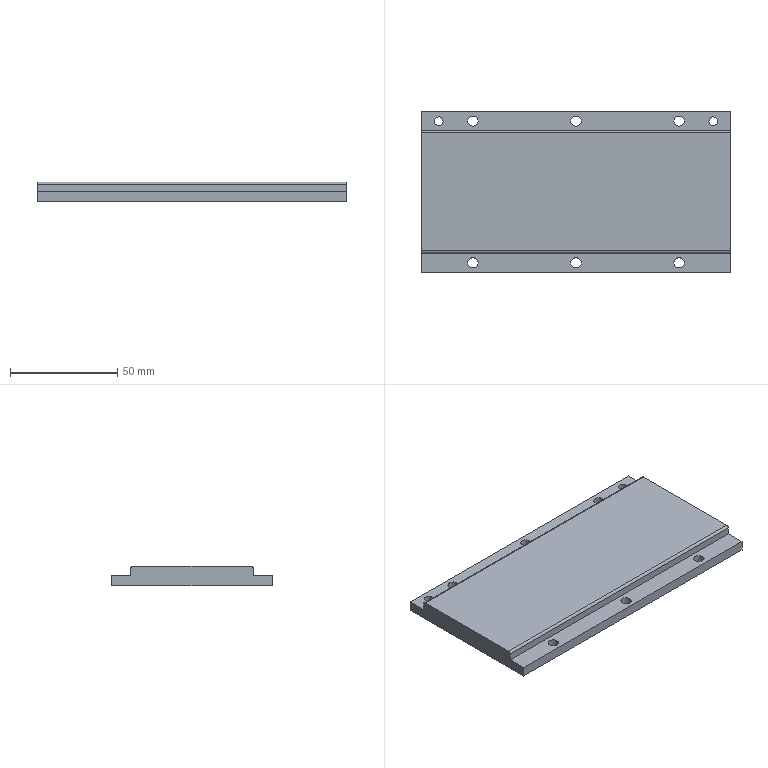Part | NX | features BREP 1 | 1 solid | 28 faces | box 143.8 x 75 x 9.2 mm | volume 87123 mm3 | cylinder 18 | plane 10 | commonest cylinder face diameters 4.8 x12 4.1 x4 2 x2
STEP:
#1=CARTESIAN_POINT('',(133.85,33.,2.4));
#2=VERTEX_POINT('',#1);
#3=CARTESIAN_POINT('',(133.85,33.,-2.4));
#4=VERTEX_POINT('',#3);
#5=CARTESIAN_POINT('',(133.85,33.,2.4));
#6=DIRECTION('',(0.,0.,1.));
#7=VECTOR('',#6,1000.);
#8=LINE('',#5,#7);
#9=EDGE_CURVE('',#2,#4,#8,.F.);
#10=ORIENTED_EDGE('',*,*,#9,.T.);
#11=CARTESIAN_POINT('',(137.95,33.,-2.4));
#12=VERTEX_POINT('',#11);
#13=CARTESIAN_POINT('',(135.9,33.,-2.4));
#14=DIRECTION('',(0.,0.,1.));
#15=DIRECTION('',(1.,0.,0.));
#16=AXIS2_PLACEMENT_3D('',#13,#14,#15);
#17=CIRCLE('',#16,2.05);
#18=EDGE_CURVE('',#12,#4,#17,.T.);
#19=ORIENTED_EDGE('',*,*,#18,.F.);
#20=CARTESIAN_POINT('',(137.95,33.,2.4));
#21=VERTEX_POINT('',#20);
#22=CARTESIAN_POINT('',(137.95,33.,2.4));
#23=DIRECTION('',(0.,0.,1.));
#24=VECTOR('',#23,1000.);
#25=LINE('',#22,#24);
#26=EDGE_CURVE('',#21,#12,#25,.F.);
#27=ORIENTED_EDGE('',*,*,#26,.F.);
#28=CARTESIAN_POINT('',(135.9,33.,2.4));
#29=DIRECTION('',(0.,0.,1.));
#30=DIRECTION('',(1.,0.,0.));
#31=AXIS2_PLACEMENT_3D('',#28,#29,#30);
#32=CIRCLE('',#31,2.05);
#33=EDGE_CURVE('',#21,#2,#32,.T.);
#34=ORIENTED_EDGE('',*,*,#33,.T.);
#35=EDGE_LOOP('',(#10,#19,#27,#34));
#36=FACE_BOUND('',#35,.T.);
#37=CARTESIAN_POINT('',(135.9,33.,2.4));
#38=DIRECTION('',(0.,0.,1.));
#39=DIRECTION('',(1.,0.,0.));
#40=AXIS2_PLACEMENT_3D('',#37,#38,#39);
#41=CYLINDRICAL_SURFACE('',#40,2.05);
#42=ADVANCED_FACE('',(#36),#41,.F.);
#43=CARTESIAN_POINT('',(5.85,33.,2.4));
#44=VERTEX_POINT('',#43);
#45=CARTESIAN_POINT('',(5.85,33.,-2.4));
#46=VERTEX_POINT('',#45);
#47=CARTESIAN_POINT('',(5.85,33.,2.4));
#48=DIRECTION('',(0.,0.,1.));
#49=VECTOR('',#48,1000.);
#50=LINE('',#47,#49);
#51=EDGE_CURVE('',#44,#46,#50,.F.);
#52=ORIENTED_EDGE('',*,*,#51,.T.);
#53=CARTESIAN_POINT('',(9.95,33.,-2.4));
#54=VERTEX_POINT('',#53);
#55=CARTESIAN_POINT('',(7.9,33.,-2.4));
#56=DIRECTION('',(0.,0.,1.));
#57=DIRECTION('',(1.,0.,0.));
#58=AXIS2_PLACEMENT_3D('',#55,#56,#57);
#59=CIRCLE('',#58,2.05);
#60=EDGE_CURVE('',#54,#46,#59,.T.);
#61=ORIENTED_EDGE('',*,*,#60,.F.);
#62=CARTESIAN_POINT('',(9.95,33.,2.4));
#63=VERTEX_POINT('',#62);
#64=CARTESIAN_POINT('',(9.95,33.,2.4));
#65=DIRECTION('',(0.,0.,1.));
#66=VECTOR('',#65,1000.);
#67=LINE('',#64,#66);
#68=EDGE_CURVE('',#63,#54,#67,.F.);
#69=ORIENTED_EDGE('',*,*,#68,.F.);
#70=CARTESIAN_POINT('',(7.9,33.,2.4));
#71=DIRECTION('',(0.,0.,1.));
#72=DIRECTION('',(1.,0.,0.));
#73=AXIS2_PLACEMENT_3D('',#70,#71,#72);
#74=CIRCLE('',#73,2.05);
#75=EDGE_CURVE('',#63,#44,#74,.T.);
#76=ORIENTED_EDGE('',*,*,#75,.T.);
#77=EDGE_LOOP('',(#52,#61,#69,#76));
#78=FACE_BOUND('',#77,.T.);
#79=CARTESIAN_POINT('',(7.9,33.,2.4));
#80=DIRECTION('',(0.,0.,1.));
#81=DIRECTION('',(1.,0.,0.));
#82=AXIS2_PLACEMENT_3D('',#79,#80,#81);
#83=CYLINDRICAL_SURFACE('',#82,2.05);
#84=ADVANCED_FACE('',(#78),#83,.F.);
#85=CARTESIAN_POINT('',(117.5,33.,2.4));
#86=VERTEX_POINT('',#85);
#87=CARTESIAN_POINT('',(117.5,33.,-2.4));
#88=VERTEX_POINT('',#87);
#89=CARTESIAN_POINT('',(117.5,33.,2.4));
#90=DIRECTION('',(0.,0.,1.));
#91=VECTOR('',#90,1000.);
#92=LINE('',#89,#91);
#93=EDGE_CURVE('',#86,#88,#92,.F.);
#94=ORIENTED_EDGE('',*,*,#93,.T.);
#95=CARTESIAN_POINT('',(122.3,33.,-2.4));
#96=VERTEX_POINT('',#95);
#97=CARTESIAN_POINT('',(119.9,33.,-2.4));
#98=DIRECTION('',(0.,0.,1.));
#99=DIRECTION('',(1.,0.,0.));
#100=AXIS2_PLACEMENT_3D('',#97,#98,#99);
#101=CIRCLE('',#100,2.4);
#102=EDGE_CURVE('',#96,#88,#101,.T.);
#103=ORIENTED_EDGE('',*,*,#102,.F.);
#104=CARTESIAN_POINT('',(122.3,33.,2.4));
#105=VERTEX_POINT('',#104);
#106=CARTESIAN_POINT('',(122.3,33.,2.4));
#107=DIRECTION('',(0.,0.,1.));
#108=VECTOR('',#107,1000.);
#109=LINE('',#106,#108);
#110=EDGE_CURVE('',#105,#96,#109,.F.);
#111=ORIENTED_EDGE('',*,*,#110,.F.);
#112=CARTESIAN_POINT('',(119.9,33.,2.4));
#113=DIRECTION('',(0.,0.,1.));
#114=DIRECTION('',(1.,0.,0.));
#115=AXIS2_PLACEMENT_3D('',#112,#113,#114);
#116=CIRCLE('',#115,2.4);
#117=EDGE_CURVE('',#105,#86,#116,.T.);
#118=ORIENTED_EDGE('',*,*,#117,.T.);
#119=EDGE_LOOP('',(#94,#103,#111,#118));
#120=FACE_BOUND('',#119,.T.);
#121=CARTESIAN_POINT('',(119.9,33.,2.4));
#122=DIRECTION('',(0.,0.,1.));
#123=DIRECTION('',(1.,0.,0.));
#124=AXIS2_PLACEMENT_3D('',#121,#122,#123);
#125=CYLINDRICAL_SURFACE('',#124,2.4);
#126=ADVANCED_FACE('',(#120),#125,.F.);
#127=CARTESIAN_POINT('',(117.5,-33.,2.4));
#128=VERTEX_POINT('',#127);
#129=CARTESIAN_POINT('',(117.5,-33.,-2.4));
#130=VERTEX_POINT('',#129);
#131=CARTESIAN_POINT('',(117.5,-33.,2.4));
#132=DIRECTION('',(0.,0.,1.));
#133=VECTOR('',#132,1000.);
#134=LINE('',#131,#133);
#135=EDGE_CURVE('',#128,#130,#134,.F.);
#136=ORIENTED_EDGE('',*,*,#135,.T.);
#137=CARTESIAN_POINT('',(122.3,-33.,-2.4));
#138=VERTEX_POINT('',#137);
#139=CARTESIAN_POINT('',(119.9,-33.,-2.4));
#140=DIRECTION('',(0.,0.,1.));
#141=DIRECTION('',(1.,0.,0.));
#142=AXIS2_PLACEMENT_3D('',#139,#140,#141);
#143=CIRCLE('',#142,2.4);
#144=EDGE_CURVE('',#138,#130,#143,.T.);
#145=ORIENTED_EDGE('',*,*,#144,.F.);
#146=CARTESIAN_POINT('',(122.3,-33.,2.4));
#147=VERTEX_POINT('',#146);
#148=CARTESIAN_POINT('',(122.3,-33.,2.4));
#149=DIRECTION('',(0.,0.,1.));
#150=VECTOR('',#149,1000.);
#151=LINE('',#148,#150);
#152=EDGE_CURVE('',#147,#138,#151,.F.);
#153=ORIENTED_EDGE('',*,*,#152,.F.);
#154=CARTESIAN_POINT('',(119.9,-33.,2.4));
#155=DIRECTION('',(0.,0.,1.));
#156=DIRECTION('',(1.,0.,0.));
#157=AXIS2_PLACEMENT_3D('',#154,#155,#156);
#158=CIRCLE('',#157,2.4);
#159=EDGE_CURVE('',#147,#128,#158,.T.);
#160=ORIENTED_EDGE('',*,*,#159,.T.);
#161=EDGE_LOOP('',(#136,#145,#153,#160));
#162=FACE_BOUND('',#161,.T.);
#163=CARTESIAN_POINT('',(119.9,-33.,2.4));
#164=DIRECTION('',(0.,0.,1.));
#165=DIRECTION('',(1.,0.,0.));
#166=AXIS2_PLACEMENT_3D('',#163,#164,#165);
#167=CYLINDRICAL_SURFACE('',#166,2.4);
#168=ADVANCED_FACE('',(#162),#167,.F.);
#169=CARTESIAN_POINT('',(69.5,33.,2.4));
#170=VERTEX_POINT('',#169);
#171=CARTESIAN_POINT('',(69.5,33.,-2.4));
#172=VERTEX_POINT('',#171);
#173=CARTESIAN_POINT('',(69.5,33.,2.4));
#174=DIRECTION('',(0.,0.,1.));
#175=VECTOR('',#174,1000.);
#176=LINE('',#173,#175);
#177=EDGE_CURVE('',#170,#172,#176,.F.);
#178=ORIENTED_EDGE('',*,*,#177,.T.);
#179=CARTESIAN_POINT('',(74.3,33.,-2.4));
#180=VERTEX_POINT('',#179);
#181=CARTESIAN_POINT('',(71.9,33.,-2.4));
#182=DIRECTION('',(0.,0.,1.));
#183=DIRECTION('',(1.,0.,0.));
#184=AXIS2_PLACEMENT_3D('',#181,#182,#183);
#185=CIRCLE('',#184,2.4);
#186=EDGE_CURVE('',#180,#172,#185,.T.);
#187=ORIENTED_EDGE('',*,*,#186,.F.);
#188=CARTESIAN_POINT('',(74.3,33.,2.4));
#189=VERTEX_POINT('',#188);
#190=CARTESIAN_POINT('',(74.3,33.,2.4));
#191=DIRECTION('',(0.,0.,1.));
#192=VECTOR('',#191,1000.);
#193=LINE('',#190,#192);
#194=EDGE_CURVE('',#189,#180,#193,.F.);
#195=ORIENTED_EDGE('',*,*,#194,.F.);
#196=CARTESIAN_POINT('',(71.9,33.,2.4));
#197=DIRECTION('',(0.,0.,1.));
#198=DIRECTION('',(1.,0.,0.));
#199=AXIS2_PLACEMENT_3D('',#196,#197,#198);
#200=CIRCLE('',#199,2.4);
#201=EDGE_CURVE('',#189,#170,#200,.T.);
#202=ORIENTED_EDGE('',*,*,#201,.T.);
#203=EDGE_LOOP('',(#178,#187,#195,#202));
#204=FACE_BOUND('',#203,.T.);
#205=CARTESIAN_POINT('',(71.9,33.,2.4));
#206=DIRECTION('',(0.,0.,1.));
#207=DIRECTION('',(1.,0.,0.));
#208=AXIS2_PLACEMENT_3D('',#205,#206,#207);
#209=CYLINDRICAL_SURFACE('',#208,2.4);
#210=ADVANCED_FACE('',(#204),#209,.F.);
#211=CARTESIAN_POINT('',(69.5,-33.,2.4));
#212=VERTEX_POINT('',#211);
#213=CARTESIAN_POINT('',(69.5,-33.,-2.4));
#214=VERTEX_POINT('',#213);
#215=CARTESIAN_POINT('',(69.5,-33.,2.4));
#216=DIRECTION('',(0.,0.,1.));
#217=VECTOR('',#216,1000.);
#218=LINE('',#215,#217);
#219=EDGE_CURVE('',#212,#214,#218,.F.);
#220=ORIENTED_EDGE('',*,*,#219,.T.);
#221=CARTESIAN_POINT('',(74.3,-33.,-2.4));
#222=VERTEX_POINT('',#221);
#223=CARTESIAN_POINT('',(71.9,-33.,-2.4));
#224=DIRECTION('',(0.,0.,1.));
#225=DIRECTION('',(1.,0.,0.));
#226=AXIS2_PLACEMENT_3D('',#223,#224,#225);
#227=CIRCLE('',#226,2.4);
#228=EDGE_CURVE('',#222,#214,#227,.T.);
#229=ORIENTED_EDGE('',*,*,#228,.F.);
#230=CARTESIAN_POINT('',(74.3,-33.,2.4));
#231=VERTEX_POINT('',#230);
#232=CARTESIAN_POINT('',(74.3,-33.,2.4));
#233=DIRECTION('',(0.,0.,1.));
#234=VECTOR('',#233,1000.);
#235=LINE('',#232,#234);
#236=EDGE_CURVE('',#231,#222,#235,.F.);
#237=ORIENTED_EDGE('',*,*,#236,.F.);
#238=CARTESIAN_POINT('',(71.9,-33.,2.4));
#239=DIRECTION('',(0.,0.,1.));
#240=DIRECTION('',(1.,0.,0.));
#241=AXIS2_PLACEMENT_3D('',#238,#239,#240);
#242=CIRCLE('',#241,2.4);
#243=EDGE_CURVE('',#231,#212,#242,.T.);
#244=ORIENTED_EDGE('',*,*,#243,.T.);
#245=EDGE_LOOP('',(#220,#229,#237,#244));
#246=FACE_BOUND('',#245,.T.);
#247=CARTESIAN_POINT('',(71.9,-33.,2.4));
#248=DIRECTION('',(0.,0.,1.));
#249=DIRECTION('',(1.,0.,0.));
#250=AXIS2_PLACEMENT_3D('',#247,#248,#249);
#251=CYLINDRICAL_SURFACE('',#250,2.4);
#252=ADVANCED_FACE('',(#246),#251,.F.);
#253=CARTESIAN_POINT('',(21.5,33.,2.4));
#254=VERTEX_POINT('',#253);
#255=CARTESIAN_POINT('',(21.5,33.,-2.4));
#256=VERTEX_POINT('',#255);
#257=CARTESIAN_POINT('',(21.5,33.,2.4));
#258=DIRECTION('',(0.,0.,1.));
#259=VECTOR('',#258,1000.);
#260=LINE('',#257,#259);
#261=EDGE_CURVE('',#254,#256,#260,.F.);
#262=ORIENTED_EDGE('',*,*,#261,.T.);
#263=CARTESIAN_POINT('',(26.3,33.,-2.4));
#264=VERTEX_POINT('',#263);
#265=CARTESIAN_POINT('',(23.9,33.,-2.4));
#266=DIRECTION('',(0.,0.,1.));
#267=DIRECTION('',(1.,0.,0.));
#268=AXIS2_PLACEMENT_3D('',#265,#266,#267);
#269=CIRCLE('',#268,2.4);
#270=EDGE_CURVE('',#264,#256,#269,.T.);
#271=ORIENTED_EDGE('',*,*,#270,.F.);
#272=CARTESIAN_POINT('',(26.3,33.,2.4));
#273=VERTEX_POINT('',#272);
#274=CARTESIAN_POINT('',(26.3,33.,2.4));
#275=DIRECTION('',(0.,0.,1.));
#276=VECTOR('',#275,1000.);
#277=LINE('',#274,#276);
#278=EDGE_CURVE('',#273,#264,#277,.F.);
#279=ORIENTED_EDGE('',*,*,#278,.F.);
#280=CARTESIAN_POINT('',(23.9,33.,2.4));
#281=DIRECTION('',(0.,0.,1.));
#282=DIRECTION('',(1.,0.,0.));
#283=AXIS2_PLACEMENT_3D('',#280,#281,#282);
#284=CIRCLE('',#283,2.4);
#285=EDGE_CURVE('',#273,#254,#284,.T.);
#286=ORIENTED_EDGE('',*,*,#285,.T.);
#287=EDGE_LOOP('',(#262,#271,#279,#286));
#288=FACE_BOUND('',#287,.T.);
#289=CARTESIAN_POINT('',(23.9,33.,2.4));
#290=DIRECTION('',(0.,0.,1.));
#291=DIRECTION('',(1.,0.,0.));
#292=AXIS2_PLACEMENT_3D('',#289,#290,#291);
#293=CYLINDRICAL_SURFACE('',#292,2.4);
#294=ADVANCED_FACE('',(#288),#293,.F.);
#295=CARTESIAN_POINT('',(21.5,-33.,2.4));
#296=VERTEX_POINT('',#295);
#297=CARTESIAN_POINT('',(21.5,-33.,-2.4));
#298=VERTEX_POINT('',#297);
#299=CARTESIAN_POINT('',(21.5,-33.,2.4));
#300=DIRECTION('',(0.,0.,1.));
#301=VECTOR('',#300,1000.);
#302=LINE('',#299,#301);
#303=EDGE_CURVE('',#296,#298,#302,.F.);
#304=ORIENTED_EDGE('',*,*,#303,.T.);
#305=CARTESIAN_POINT('',(26.3,-33.,-2.4));
#306=VERTEX_POINT('',#305);
#307=CARTESIAN_POINT('',(23.9,-33.,-2.4));
#308=DIRECTION('',(0.,0.,1.));
#309=DIRECTION('',(1.,0.,0.));
#310=AXIS2_PLACEMENT_3D('',#307,#308,#309);
#311=CIRCLE('',#310,2.4);
#312=EDGE_CURVE('',#306,#298,#311,.T.);
#313=ORIENTED_EDGE('',*,*,#312,.F.);
#314=CARTESIAN_POINT('',(26.3,-33.,2.4));
#315=VERTEX_POINT('',#314);
#316=CARTESIAN_POINT('',(26.3,-33.,2.4));
#317=DIRECTION('',(0.,0.,1.));
#318=VECTOR('',#317,1000.);
#319=LINE('',#316,#318);
#320=EDGE_CURVE('',#315,#306,#319,.F.);
#321=ORIENTED_EDGE('',*,*,#320,.F.);
#322=CARTESIAN_POINT('',(23.9,-33.,2.4));
#323=DIRECTION('',(0.,0.,1.));
#324=DIRECTION('',(1.,0.,0.));
#325=AXIS2_PLACEMENT_3D('',#322,#323,#324);
#326=CIRCLE('',#325,2.4);
#327=EDGE_CURVE('',#315,#296,#326,.T.);
#328=ORIENTED_EDGE('',*,*,#327,.T.);
#329=EDGE_LOOP('',(#304,#313,#321,#328));
#330=FACE_BOUND('',#329,.T.);
#331=CARTESIAN_POINT('',(23.9,-33.,2.4));
#332=DIRECTION('',(0.,0.,1.));
#333=DIRECTION('',(1.,0.,0.));
#334=AXIS2_PLACEMENT_3D('',#331,#332,#333);
#335=CYLINDRICAL_SURFACE('',#334,2.4);
#336=ADVANCED_FACE('',(#330),#335,.F.);
#337=CARTESIAN_POINT('',(0.,37.5,2.4));
#338=VERTEX_POINT('',#337);
#339=CARTESIAN_POINT('',(0.,28.5,2.4));
#340=VERTEX_POINT('',#339);
#341=CARTESIAN_POINT('',(0.,37.5,2.4));
#342=DIRECTION('',(0.,-1.,0.));
#343=VECTOR('',#342,1000.);
#344=LINE('',#341,#343);
#345=EDGE_CURVE('',#338,#340,#344,.T.);
#346=ORIENTED_EDGE('',*,*,#345,.F.);
#347=CARTESIAN_POINT('',(0.,37.5,-2.4));
#348=VERTEX_POINT('',#347);
#349=CARTESIAN_POINT('',(0.,37.5,-2.4));
#350=DIRECTION('',(0.,0.,1.));
#351=VECTOR('',#350,1000.);
#352=LINE('',#349,#351);
#353=EDGE_CURVE('',#348,#338,#352,.T.);
#354=ORIENTED_EDGE('',*,*,#353,.F.);
#355=CARTESIAN_POINT('',(0.,-37.5,-2.4));
#356=VERTEX_POINT('',#355);
#357=CARTESIAN_POINT('',(0.,-37.5,-2.4));
#358=DIRECTION('',(0.,1.,0.));
#359=VECTOR('',#358,1000.);
#360=LINE('',#357,#359);
#361=EDGE_CURVE('',#356,#348,#360,.T.);
#362=ORIENTED_EDGE('',*,*,#361,.F.);
#363=CARTESIAN_POINT('',(0.,-37.5,2.4));
#364=VERTEX_POINT('',#363);
#365=CARTESIAN_POINT('',(0.,-37.5,2.4));
#366=DIRECTION('',(0.,0.,-1.));
#367=VECTOR('',#366,1000.);
#368=LINE('',#365,#367);
#369=EDGE_CURVE('',#364,#356,#368,.T.);
#370=ORIENTED_EDGE('',*,*,#369,.F.);
#371=CARTESIAN_POINT('',(0.,-28.5,2.4));
#372=VERTEX_POINT('',#371);
#373=CARTESIAN_POINT('',(0.,-28.5,2.4));
#374=DIRECTION('',(0.,-1.,0.));
#375=VECTOR('',#374,1000.);
#376=LINE('',#373,#375);
#377=EDGE_CURVE('',#372,#364,#376,.T.);
#378=ORIENTED_EDGE('',*,*,#377,.F.);
#379=CARTESIAN_POINT('',(0.,-28.5,5.8));
#380=VERTEX_POINT('',#379);
#381=CARTESIAN_POINT('',(0.,-28.5,5.8));
#382=DIRECTION('',(0.,0.,-1.));
#383=VECTOR('',#382,1000.);
#384=LINE('',#381,#383);
#385=EDGE_CURVE('',#380,#372,#384,.T.);
#386=ORIENTED_EDGE('',*,*,#385,.F.);
#387=CARTESIAN_POINT('',(0.,-27.5,6.8));
#388=VERTEX_POINT('',#387);
#389=CARTESIAN_POINT('',(0.,-27.5,5.8));
#390=DIRECTION('',(1.,0.,0.));
#391=DIRECTION('',(0.,0.,-1.));
#392=AXIS2_PLACEMENT_3D('',#389,#390,#391);
#393=CIRCLE('',#392,1.);
#394=EDGE_CURVE('',#388,#380,#393,.T.);
#395=ORIENTED_EDGE('',*,*,#394,.F.);
#396=CARTESIAN_POINT('',(0.,27.5,6.8));
#397=VERTEX_POINT('',#396);
#398=CARTESIAN_POINT('',(0.,27.5,6.8));
#399=DIRECTION('',(0.,-1.,0.));
#400=VECTOR('',#399,1000.);
#401=LINE('',#398,#400);
#402=EDGE_CURVE('',#397,#388,#401,.T.);
#403=ORIENTED_EDGE('',*,*,#402,.F.);
#404=CARTESIAN_POINT('',(0.,28.5,5.8));
#405=VERTEX_POINT('',#404);
#406=CARTESIAN_POINT('',(0.,27.5,5.8));
#407=DIRECTION('',(1.,0.,0.));
#408=DIRECTION('',(0.,0.,-1.));
#409=AXIS2_PLACEMENT_3D('',#406,#407,#408);
#410=CIRCLE('',#409,1.);
#411=EDGE_CURVE('',#405,#397,#410,.T.);
#412=ORIENTED_EDGE('',*,*,#411,.F.);
#413=CARTESIAN_POINT('',(0.,28.5,2.4));
#414=DIRECTION('',(0.,0.,1.));
#415=VECTOR('',#414,1000.);
#416=LINE('',#413,#415);
#417=EDGE_CURVE('',#340,#405,#416,.T.);
#418=ORIENTED_EDGE('',*,*,#417,.F.);
#419=EDGE_LOOP('',(#346,#354,#362,#370,#378,#386,#395,#403,#412,#418));
#420=FACE_BOUND('',#419,.T.);
#421=CARTESIAN_POINT('',(0.,27.5,5.8));
#422=DIRECTION('',(1.,0.,0.));
#423=DIRECTION('',(0.,0.,-1.));
#424=AXIS2_PLACEMENT_3D('',#421,#422,#423);
#425=PLANE('',#424);
#426=ADVANCED_FACE('',(#420),#425,.F.);
#427=CARTESIAN_POINT('',(143.8,37.5,2.4));
#428=VERTEX_POINT('',#427);
#429=CARTESIAN_POINT('',(143.8,28.5,2.4));
#430=VERTEX_POINT('',#429);
#431=CARTESIAN_POINT('',(143.8,37.5,2.4));
#432=DIRECTION('',(0.,-1.,0.));
#433=VECTOR('',#432,1000.);
#434=LINE('',#431,#433);
#435=EDGE_CURVE('',#428,#430,#434,.T.);
#436=ORIENTED_EDGE('',*,*,#435,.T.);
#437=CARTESIAN_POINT('',(143.8,28.5,5.8));
#438=VERTEX_POINT('',#437);
#439=CARTESIAN_POINT('',(143.8,28.5,2.4));
#440=DIRECTION('',(0.,0.,1.));
#441=VECTOR('',#440,1000.);
#442=LINE('',#439,#441);
#443=EDGE_CURVE('',#430,#438,#442,.T.);
#444=ORIENTED_EDGE('',*,*,#443,.T.);
#445=CARTESIAN_POINT('',(143.8,27.5,6.8));
#446=VERTEX_POINT('',#445);
#447=CARTESIAN_POINT('',(143.8,27.5,5.8));
#448=DIRECTION('',(1.,0.,0.));
#449=DIRECTION('',(0.,0.,-1.));
#450=AXIS2_PLACEMENT_3D('',#447,#448,#449);
#451=CIRCLE('',#450,1.);
#452=EDGE_CURVE('',#438,#446,#451,.T.);
#453=ORIENTED_EDGE('',*,*,#452,.T.);
#454=CARTESIAN_POINT('',(143.8,-27.5,6.8));
#455=VERTEX_POINT('',#454);
#456=CARTESIAN_POINT('',(143.8,27.5,6.8));
#457=DIRECTION('',(0.,-1.,0.));
#458=VECTOR('',#457,1000.);
#459=LINE('',#456,#458);
#460=EDGE_CURVE('',#446,#455,#459,.T.);
#461=ORIENTED_EDGE('',*,*,#460,.T.);
#462=CARTESIAN_POINT('',(143.8,-28.5,5.8));
#463=VERTEX_POINT('',#462);
#464=CARTESIAN_POINT('',(143.8,-27.5,5.8));
#465=DIRECTION('',(1.,0.,0.));
#466=DIRECTION('',(0.,0.,-1.));
#467=AXIS2_PLACEMENT_3D('',#464,#465,#466);
#468=CIRCLE('',#467,1.);
#469=EDGE_CURVE('',#455,#463,#468,.T.);
#470=ORIENTED_EDGE('',*,*,#469,.T.);
#471=CARTESIAN_POINT('',(143.8,-28.5,2.4));
#472=VERTEX_POINT('',#471);
#473=CARTESIAN_POINT('',(143.8,-28.5,5.8));
#474=DIRECTION('',(0.,0.,-1.));
#475=VECTOR('',#474,1000.);
#476=LINE('',#473,#475);
#477=EDGE_CURVE('',#463,#472,#476,.T.);
#478=ORIENTED_EDGE('',*,*,#477,.T.);
#479=CARTESIAN_POINT('',(143.8,-37.5,2.4));
#480=VERTEX_POINT('',#479);
#481=CARTESIAN_POINT('',(143.8,-28.5,2.4));
#482=DIRECTION('',(0.,-1.,0.));
#483=VECTOR('',#482,1000.);
#484=LINE('',#481,#483);
#485=EDGE_CURVE('',#472,#480,#484,.T.);
#486=ORIENTED_EDGE('',*,*,#485,.T.);
#487=CARTESIAN_POINT('',(143.8,-37.5,-2.4));
#488=VERTEX_POINT('',#487);
#489=CARTESIAN_POINT('',(143.8,-37.5,2.4));
#490=DIRECTION('',(0.,0.,-1.));
#491=VECTOR('',#490,1000.);
#492=LINE('',#489,#491);
#493=EDGE_CURVE('',#480,#488,#492,.T.);
#494=ORIENTED_EDGE('',*,*,#493,.T.);
#495=CARTESIAN_POINT('',(143.8,37.5,-2.4));
#496=VERTEX_POINT('',#495);
#497=CARTESIAN_POINT('',(143.8,-37.5,-2.4));
#498=DIRECTION('',(0.,1.,0.));
#499=VECTOR('',#498,1000.);
#500=LINE('',#497,#499);
#501=EDGE_CURVE('',#488,#496,#500,.T.);
#502=ORIENTED_EDGE('',*,*,#501,.T.);
#503=CARTESIAN_POINT('',(143.8,37.5,-2.4));
#504=DIRECTION('',(0.,0.,1.));
#505=VECTOR('',#504,1000.);
#506=LINE('',#503,#505);
#507=EDGE_CURVE('',#496,#428,#506,.T.);
#508=ORIENTED_EDGE('',*,*,#507,.T.);
#509=EDGE_LOOP('',(#436,#444,#453,#461,#470,#478,#486,#494,#502,#508));
#510=FACE_BOUND('',#509,.T.);
#511=CARTESIAN_POINT('',(143.8,27.5,5.8));
#512=DIRECTION('',(1.,0.,0.));
#513=DIRECTION('',(0.,0.,-1.));
#514=AXIS2_PLACEMENT_3D('',#511,#512,#513);
#515=PLANE('',#514);
#516=ADVANCED_FACE('',(#510),#515,.T.);
#517=ORIENTED_EDGE('',*,*,#353,.T.);
#518=CARTESIAN_POINT('',(143.8,37.5,2.4));
#519=DIRECTION('',(-1.,0.,0.));
#520=VECTOR('',#519,1000.);
#521=LINE('',#518,#520);
#522=EDGE_CURVE('',#428,#338,#521,.T.);
#523=ORIENTED_EDGE('',*,*,#522,.F.);
#524=ORIENTED_EDGE('',*,*,#507,.F.);
#525=CARTESIAN_POINT('',(143.8,37.5,-2.4));
#526=DIRECTION('',(-1.,0.,0.));
#527=VECTOR('',#526,1000.);
#528=LINE('',#525,#527);
#529=EDGE_CURVE('',#496,#348,#528,.T.);
#530=ORIENTED_EDGE('',*,*,#529,.T.);
#531=EDGE_LOOP('',(#517,#523,#524,#530));
#532=FACE_BOUND('',#531,.T.);
#533=CARTESIAN_POINT('',(143.8,37.5,-2.4));
#534=DIRECTION('',(0.,-1.,0.));
#535=DIRECTION('',(0.,0.,-1.));
#536=AXIS2_PLACEMENT_3D('',#533,#534,#535);
#537=PLANE('',#536);
#538=ADVANCED_FACE('',(#532),#537,.F.);
#539=ORIENTED_EDGE('',*,*,#361,.T.);
#540=ORIENTED_EDGE('',*,*,#529,.F.);
#541=ORIENTED_EDGE('',*,*,#501,.F.);
#542=CARTESIAN_POINT('',(143.8,-37.5,-2.4));
#543=DIRECTION('',(-1.,0.,0.));
#544=VECTOR('',#543,1000.);
#545=LINE('',#542,#544);
#546=EDGE_CURVE('',#488,#356,#545,.T.);
#547=ORIENTED_EDGE('',*,*,#546,.T.);
#548=EDGE_LOOP('',(#539,#540,#541,#547));
#549=FACE_BOUND('',#548,.T.);
#550=ORIENTED_EDGE('',*,*,#312,.T.);
#551=CARTESIAN_POINT('',(23.9,-33.,-2.4));
#552=DIRECTION('',(0.,0.,1.));
#553=DIRECTION('',(1.,0.,0.));
#554=AXIS2_PLACEMENT_3D('',#551,#552,#553);
#555=CIRCLE('',#554,2.4);
#556=EDGE_CURVE('',#298,#306,#555,.T.);
#557=ORIENTED_EDGE('',*,*,#556,.T.);
#558=EDGE_LOOP('',(#550,#557));
#559=FACE_BOUND('',#558,.T.);
#560=ORIENTED_EDGE('',*,*,#270,.T.);
#561=CARTESIAN_POINT('',(23.9,33.,-2.4));
#562=DIRECTION('',(0.,0.,1.));
#563=DIRECTION('',(1.,0.,0.));
#564=AXIS2_PLACEMENT_3D('',#561,#562,#563);
#565=CIRCLE('',#564,2.4);
#566=EDGE_CURVE('',#256,#264,#565,.T.);
#567=ORIENTED_EDGE('',*,*,#566,.T.);
#568=EDGE_LOOP('',(#560,#567));
#569=FACE_BOUND('',#568,.T.);
#570=ORIENTED_EDGE('',*,*,#228,.T.);
#571=CARTESIAN_POINT('',(71.9,-33.,-2.4));
#572=DIRECTION('',(0.,0.,1.));
#573=DIRECTION('',(1.,0.,0.));
#574=AXIS2_PLACEMENT_3D('',#571,#572,#573);
#575=CIRCLE('',#574,2.4);
#576=EDGE_CURVE('',#214,#222,#575,.T.);
#577=ORIENTED_EDGE('',*,*,#576,.T.);
#578=EDGE_LOOP('',(#570,#577));
#579=FACE_BOUND('',#578,.T.);
#580=ORIENTED_EDGE('',*,*,#186,.T.);
#581=CARTESIAN_POINT('',(71.9,33.,-2.4));
#582=DIRECTION('',(0.,0.,1.));
#583=DIRECTION('',(1.,0.,0.));
#584=AXIS2_PLACEMENT_3D('',#581,#582,#583);
#585=CIRCLE('',#584,2.4);
#586=EDGE_CURVE('',#172,#180,#585,.T.);
#587=ORIENTED_EDGE('',*,*,#586,.T.);
#588=EDGE_LOOP('',(#580,#587));
#589=FACE_BOUND('',#588,.T.);
#590=ORIENTED_EDGE('',*,*,#144,.T.);
#591=CARTESIAN_POINT('',(119.9,-33.,-2.4));
#592=DIRECTION('',(0.,0.,1.));
#593=DIRECTION('',(1.,0.,0.));
#594=AXIS2_PLACEMENT_3D('',#591,#592,#593);
#595=CIRCLE('',#594,2.4);
#596=EDGE_CURVE('',#130,#138,#595,.T.);
#597=ORIENTED_EDGE('',*,*,#596,.T.);
#598=EDGE_LOOP('',(#590,#597));
#599=FACE_BOUND('',#598,.T.);
#600=ORIENTED_EDGE('',*,*,#102,.T.);
#601=CARTESIAN_POINT('',(119.9,33.,-2.4));
#602=DIRECTION('',(0.,0.,1.));
#603=DIRECTION('',(1.,0.,0.));
#604=AXIS2_PLACEMENT_3D('',#601,#602,#603);
#605=CIRCLE('',#604,2.4);
#606=EDGE_CURVE('',#88,#96,#605,.T.);
#607=ORIENTED_EDGE('',*,*,#606,.T.);
#608=EDGE_LOOP('',(#600,#607));
#609=FACE_BOUND('',#608,.T.);
#610=ORIENTED_EDGE('',*,*,#60,.T.);
#611=CARTESIAN_POINT('',(7.9,33.,-2.4));
#612=DIRECTION('',(0.,0.,1.));
#613=DIRECTION('',(1.,0.,0.));
#614=AXIS2_PLACEMENT_3D('',#611,#612,#613);
#615=CIRCLE('',#614,2.05);
#616=EDGE_CURVE('',#46,#54,#615,.T.);
#617=ORIENTED_EDGE('',*,*,#616,.T.);
#618=EDGE_LOOP('',(#610,#617));
#619=FACE_BOUND('',#618,.T.);
#620=ORIENTED_EDGE('',*,*,#18,.T.);
#621=CARTESIAN_POINT('',(135.9,33.,-2.4));
#622=DIRECTION('',(0.,0.,1.));
#623=DIRECTION('',(1.,0.,0.));
#624=AXIS2_PLACEMENT_3D('',#621,#622,#623);
#625=CIRCLE('',#624,2.05);
#626=EDGE_CURVE('',#4,#12,#625,.T.);
#627=ORIENTED_EDGE('',*,*,#626,.T.);
#628=EDGE_LOOP('',(#620,#627));
#629=FACE_BOUND('',#628,.T.);
#630=CARTESIAN_POINT('',(143.8,-37.5,-2.4));
#631=DIRECTION('',(0.,0.,1.));
#632=DIRECTION('',(1.,0.,0.));
#633=AXIS2_PLACEMENT_3D('',#630,#631,#632);
#634=PLANE('',#633);
#635=ADVANCED_FACE('',(#549,#559,#569,#579,#589,#599,#609,#619,#629),#634,.F.);
#636=ORIENTED_EDGE('',*,*,#369,.T.);
#637=ORIENTED_EDGE('',*,*,#546,.F.);
#638=ORIENTED_EDGE('',*,*,#493,.F.);
#639=CARTESIAN_POINT('',(143.8,-37.5,2.4));
#640=DIRECTION('',(-1.,0.,0.));
#641=VECTOR('',#640,1000.);
#642=LINE('',#639,#641);
#643=EDGE_CURVE('',#480,#364,#642,.T.);
#644=ORIENTED_EDGE('',*,*,#643,.T.);
#645=EDGE_LOOP('',(#636,#637,#638,#644));
#646=FACE_BOUND('',#645,.T.);
#647=CARTESIAN_POINT('',(143.8,-37.5,2.4));
#648=DIRECTION('',(0.,1.,0.));
#649=DIRECTION('',(0.,0.,1.));
#650=AXIS2_PLACEMENT_3D('',#647,#648,#649);
#651=PLANE('',#650);
#652=ADVANCED_FACE('',(#646),#651,.F.);
#653=ORIENTED_EDGE('',*,*,#377,.T.);
#654=ORIENTED_EDGE('',*,*,#643,.F.);
#655=ORIENTED_EDGE('',*,*,#485,.F.);
#656=CARTESIAN_POINT('',(143.8,-28.5,2.4));
#657=DIRECTION('',(-1.,0.,0.));
#658=VECTOR('',#657,1000.);
#659=LINE('',#656,#658);
#660=EDGE_CURVE('',#472,#372,#659,.T.);
#661=ORIENTED_EDGE('',*,*,#660,.T.);
#662=EDGE_LOOP('',(#653,#654,#655,#661));
#663=FACE_BOUND('',#662,.T.);
#664=ORIENTED_EDGE('',*,*,#327,.F.);
#665=CARTESIAN_POINT('',(23.9,-33.,2.4));
#666=DIRECTION('',(0.,0.,1.));
#667=DIRECTION('',(1.,0.,0.));
#668=AXIS2_PLACEMENT_3D('',#665,#666,#667);
#669=CIRCLE('',#668,2.4);
#670=EDGE_CURVE('',#296,#315,#669,.T.);
#671=ORIENTED_EDGE('',*,*,#670,.F.);
#672=EDGE_LOOP('',(#664,#671));
#673=FACE_BOUND('',#672,.T.);
#674=ORIENTED_EDGE('',*,*,#243,.F.);
#675=CARTESIAN_POINT('',(71.9,-33.,2.4));
#676=DIRECTION('',(0.,0.,1.));
#677=DIRECTION('',(1.,0.,0.));
#678=AXIS2_PLACEMENT_3D('',#675,#676,#677);
#679=CIRCLE('',#678,2.4);
#680=EDGE_CURVE('',#212,#231,#679,.T.);
#681=ORIENTED_EDGE('',*,*,#680,.F.);
#682=EDGE_LOOP('',(#674,#681));
#683=FACE_BOUND('',#682,.T.);
#684=ORIENTED_EDGE('',*,*,#159,.F.);
#685=CARTESIAN_POINT('',(119.9,-33.,2.4));
#686=DIRECTION('',(0.,0.,1.));
#687=DIRECTION('',(1.,0.,0.));
#688=AXIS2_PLACEMENT_3D('',#685,#686,#687);
#689=CIRCLE('',#688,2.4);
#690=EDGE_CURVE('',#128,#147,#689,.T.);
#691=ORIENTED_EDGE('',*,*,#690,.F.);
#692=EDGE_LOOP('',(#684,#691));
#693=FACE_BOUND('',#692,.T.);
#694=CARTESIAN_POINT('',(143.8,-28.5,2.4));
#695=DIRECTION('',(0.,0.,-1.));
#696=DIRECTION('',(-1.,0.,0.));
#697=AXIS2_PLACEMENT_3D('',#694,#695,#696);
#698=PLANE('',#697);
#699=ADVANCED_FACE('',(#663,#673,#683,#693),#698,.F.);
#700=ORIENTED_EDGE('',*,*,#385,.T.);
#701=ORIENTED_EDGE('',*,*,#660,.F.);
#702=ORIENTED_EDGE('',*,*,#477,.F.);
#703=CARTESIAN_POINT('',(143.8,-28.5,5.8));
#704=DIRECTION('',(-1.,0.,0.));
#705=VECTOR('',#704,1000.);
#706=LINE('',#703,#705);
#707=EDGE_CURVE('',#463,#380,#706,.T.);
#708=ORIENTED_EDGE('',*,*,#707,.T.);
#709=EDGE_LOOP('',(#700,#701,#702,#708));
#710=FACE_BOUND('',#709,.T.);
#711=CARTESIAN_POINT('',(143.8,-28.5,5.8));
#712=DIRECTION('',(0.,1.,0.));
#713=DIRECTION('',(0.,0.,1.));
#714=AXIS2_PLACEMENT_3D('',#711,#712,#713);
#715=PLANE('',#714);
#716=ADVANCED_FACE('',(#710),#715,.F.);
#717=ORIENTED_EDGE('',*,*,#394,.T.);
#718=ORIENTED_EDGE('',*,*,#707,.F.);
#719=ORIENTED_EDGE('',*,*,#469,.F.);
#720=CARTESIAN_POINT('',(143.8,-27.5,6.8));
#721=DIRECTION('',(-1.,0.,0.));
#722=VECTOR('',#721,1000.);
#723=LINE('',#720,#722);
#724=EDGE_CURVE('',#455,#388,#723,.T.);
#725=ORIENTED_EDGE('',*,*,#724,.T.);
#726=EDGE_LOOP('',(#717,#718,#719,#725));
#727=FACE_BOUND('',#726,.T.);
#728=CARTESIAN_POINT('',(143.8,-27.5,5.8));
#729=DIRECTION('',(-1.,0.,0.));
#730=DIRECTION('',(0.,0.,1.));
#731=AXIS2_PLACEMENT_3D('',#728,#729,#730);
#732=CYLINDRICAL_SURFACE('',#731,1.);
#733=ADVANCED_FACE('',(#727),#732,.T.);
#734=ORIENTED_EDGE('',*,*,#402,.T.);
#735=ORIENTED_EDGE('',*,*,#724,.F.);
#736=ORIENTED_EDGE('',*,*,#460,.F.);
#737=CARTESIAN_POINT('',(143.8,27.5,6.8));
#738=DIRECTION('',(-1.,0.,0.));
#739=VECTOR('',#738,1000.);
#740=LINE('',#737,#739);
#741=EDGE_CURVE('',#446,#397,#740,.T.);
#742=ORIENTED_EDGE('',*,*,#741,.T.);
#743=EDGE_LOOP('',(#734,#735,#736,#742));
#744=FACE_BOUND('',#743,.T.);
#745=CARTESIAN_POINT('',(143.8,27.5,6.8));
#746=DIRECTION('',(0.,0.,-1.));
#747=DIRECTION('',(-1.,0.,0.));
#748=AXIS2_PLACEMENT_3D('',#745,#746,#747);
#749=PLANE('',#748);
#750=ADVANCED_FACE('',(#744),#749,.F.);
#751=ORIENTED_EDGE('',*,*,#411,.T.);
#752=ORIENTED_EDGE('',*,*,#741,.F.);
#753=ORIENTED_EDGE('',*,*,#452,.F.);
#754=CARTESIAN_POINT('',(143.8,28.5,5.8));
#755=DIRECTION('',(-1.,0.,0.));
#756=VECTOR('',#755,1000.);
#757=LINE('',#754,#756);
#758=EDGE_CURVE('',#438,#405,#757,.T.);
#759=ORIENTED_EDGE('',*,*,#758,.T.);
#760=EDGE_LOOP('',(#751,#752,#753,#759));
#761=FACE_BOUND('',#760,.T.);
#762=CARTESIAN_POINT('',(143.8,27.5,5.8));
#763=DIRECTION('',(-1.,0.,0.));
#764=DIRECTION('',(0.,0.,1.));
#765=AXIS2_PLACEMENT_3D('',#762,#763,#764);
#766=CYLINDRICAL_SURFACE('',#765,1.);
#767=ADVANCED_FACE('',(#761),#766,.T.);
#768=ORIENTED_EDGE('',*,*,#417,.T.);
#769=ORIENTED_EDGE('',*,*,#758,.F.);
#770=ORIENTED_EDGE('',*,*,#443,.F.);
#771=CARTESIAN_POINT('',(143.8,28.5,2.4));
#772=DIRECTION('',(-1.,0.,0.));
#773=VECTOR('',#772,1000.);
#774=LINE('',#771,#773);
#775=EDGE_CURVE('',#430,#340,#774,.T.);
#776=ORIENTED_EDGE('',*,*,#775,.T.);
#777=EDGE_LOOP('',(#768,#769,#770,#776));
#778=FACE_BOUND('',#777,.T.);
#779=CARTESIAN_POINT('',(143.8,28.5,2.4));
#780=DIRECTION('',(0.,-1.,0.));
#781=DIRECTION('',(0.,0.,-1.));
#782=AXIS2_PLACEMENT_3D('',#779,#780,#781);
#783=PLANE('',#782);
#784=ADVANCED_FACE('',(#778),#783,.F.);
#785=ORIENTED_EDGE('',*,*,#345,.T.);
#786=ORIENTED_EDGE('',*,*,#775,.F.);
#787=ORIENTED_EDGE('',*,*,#435,.F.);
#788=ORIENTED_EDGE('',*,*,#522,.T.);
#789=EDGE_LOOP('',(#785,#786,#787,#788));
#790=FACE_BOUND('',#789,.T.);
#791=ORIENTED_EDGE('',*,*,#285,.F.);
#792=CARTESIAN_POINT('',(23.9,33.,2.4));
#793=DIRECTION('',(0.,0.,1.));
#794=DIRECTION('',(1.,0.,0.));
#795=AXIS2_PLACEMENT_3D('',#792,#793,#794);
#796=CIRCLE('',#795,2.4);
#797=EDGE_CURVE('',#254,#273,#796,.T.);
#798=ORIENTED_EDGE('',*,*,#797,.F.);
#799=EDGE_LOOP('',(#791,#798));
#800=FACE_BOUND('',#799,.T.);
#801=ORIENTED_EDGE('',*,*,#201,.F.);
#802=CARTESIAN_POINT('',(71.9,33.,2.4));
#803=DIRECTION('',(0.,0.,1.));
#804=DIRECTION('',(1.,0.,0.));
#805=AXIS2_PLACEMENT_3D('',#802,#803,#804);
#806=CIRCLE('',#805,2.4);
#807=EDGE_CURVE('',#170,#189,#806,.T.);
#808=ORIENTED_EDGE('',*,*,#807,.F.);
#809=EDGE_LOOP('',(#801,#808));
#810=FACE_BOUND('',#809,.T.);
#811=ORIENTED_EDGE('',*,*,#117,.F.);
#812=CARTESIAN_POINT('',(119.9,33.,2.4));
#813=DIRECTION('',(0.,0.,1.));
#814=DIRECTION('',(1.,0.,0.));
#815=AXIS2_PLACEMENT_3D('',#812,#813,#814);
#816=CIRCLE('',#815,2.4);
#817=EDGE_CURVE('',#86,#105,#816,.T.);
#818=ORIENTED_EDGE('',*,*,#817,.F.);
#819=EDGE_LOOP('',(#811,#818));
#820=FACE_BOUND('',#819,.T.);
#821=ORIENTED_EDGE('',*,*,#75,.F.);
#822=CARTESIAN_POINT('',(7.9,33.,2.4));
#823=DIRECTION('',(0.,0.,1.));
#824=DIRECTION('',(1.,0.,0.));
#825=AXIS2_PLACEMENT_3D('',#822,#823,#824);
#826=CIRCLE('',#825,2.05);
#827=EDGE_CURVE('',#44,#63,#826,.T.);
#828=ORIENTED_EDGE('',*,*,#827,.F.);
#829=EDGE_LOOP('',(#821,#828));
#830=FACE_BOUND('',#829,.T.);
#831=ORIENTED_EDGE('',*,*,#33,.F.);
#832=CARTESIAN_POINT('',(135.9,33.,2.4));
#833=DIRECTION('',(0.,0.,1.));
#834=DIRECTION('',(1.,0.,0.));
#835=AXIS2_PLACEMENT_3D('',#832,#833,#834);
#836=CIRCLE('',#835,2.05);
#837=EDGE_CURVE('',#2,#21,#836,.T.);
#838=ORIENTED_EDGE('',*,*,#837,.F.);
#839=EDGE_LOOP('',(#831,#838));
#840=FACE_BOUND('',#839,.T.);
#841=CARTESIAN_POINT('',(143.8,37.5,2.4));
#842=DIRECTION('',(0.,0.,-1.));
#843=DIRECTION('',(-1.,0.,0.));
#844=AXIS2_PLACEMENT_3D('',#841,#842,#843);
#845=PLANE('',#844);
#846=ADVANCED_FACE('',(#790,#800,#810,#820,#830,#840),#845,.F.);
#847=ORIENTED_EDGE('',*,*,#556,.F.);
#848=ORIENTED_EDGE('',*,*,#303,.F.);
#849=ORIENTED_EDGE('',*,*,#670,.T.);
#850=ORIENTED_EDGE('',*,*,#320,.T.);
#851=EDGE_LOOP('',(#847,#848,#849,#850));
#852=FACE_BOUND('',#851,.T.);
#853=CARTESIAN_POINT('',(23.9,-33.,2.4));
#854=DIRECTION('',(0.,0.,1.));
#855=DIRECTION('',(1.,0.,0.));
#856=AXIS2_PLACEMENT_3D('',#853,#854,#855);
#857=CYLINDRICAL_SURFACE('',#856,2.4);
#858=ADVANCED_FACE('',(#852),#857,.F.);
#859=ORIENTED_EDGE('',*,*,#566,.F.);
#860=ORIENTED_EDGE('',*,*,#261,.F.);
#861=ORIENTED_EDGE('',*,*,#797,.T.);
#862=ORIENTED_EDGE('',*,*,#278,.T.);
#863=EDGE_LOOP('',(#859,#860,#861,#862));
#864=FACE_BOUND('',#863,.T.);
#865=CARTESIAN_POINT('',(23.9,33.,2.4));
#866=DIRECTION('',(0.,0.,1.));
#867=DIRECTION('',(1.,0.,0.));
#868=AXIS2_PLACEMENT_3D('',#865,#866,#867);
#869=CYLINDRICAL_SURFACE('',#868,2.4);
#870=ADVANCED_FACE('',(#864),#869,.F.);
#871=ORIENTED_EDGE('',*,*,#576,.F.);
#872=ORIENTED_EDGE('',*,*,#219,.F.);
#873=ORIENTED_EDGE('',*,*,#680,.T.);
#874=ORIENTED_EDGE('',*,*,#236,.T.);
#875=EDGE_LOOP('',(#871,#872,#873,#874));
#876=FACE_BOUND('',#875,.T.);
#877=CARTESIAN_POINT('',(71.9,-33.,2.4));
#878=DIRECTION('',(0.,0.,1.));
#879=DIRECTION('',(1.,0.,0.));
#880=AXIS2_PLACEMENT_3D('',#877,#878,#879);
#881=CYLINDRICAL_SURFACE('',#880,2.4);
#882=ADVANCED_FACE('',(#876),#881,.F.);
#883=ORIENTED_EDGE('',*,*,#586,.F.);
#884=ORIENTED_EDGE('',*,*,#177,.F.);
#885=ORIENTED_EDGE('',*,*,#807,.T.);
#886=ORIENTED_EDGE('',*,*,#194,.T.);
#887=EDGE_LOOP('',(#883,#884,#885,#886));
#888=FACE_BOUND('',#887,.T.);
#889=CARTESIAN_POINT('',(71.9,33.,2.4));
#890=DIRECTION('',(0.,0.,1.));
#891=DIRECTION('',(1.,0.,0.));
#892=AXIS2_PLACEMENT_3D('',#889,#890,#891);
#893=CYLINDRICAL_SURFACE('',#892,2.4);
#894=ADVANCED_FACE('',(#888),#893,.F.);
#895=ORIENTED_EDGE('',*,*,#596,.F.);
#896=ORIENTED_EDGE('',*,*,#135,.F.);
#897=ORIENTED_EDGE('',*,*,#690,.T.);
#898=ORIENTED_EDGE('',*,*,#152,.T.);
#899=EDGE_LOOP('',(#895,#896,#897,#898));
#900=FACE_BOUND('',#899,.T.);
#901=CARTESIAN_POINT('',(119.9,-33.,2.4));
#902=DIRECTION('',(0.,0.,1.));
#903=DIRECTION('',(1.,0.,0.));
#904=AXIS2_PLACEMENT_3D('',#901,#902,#903);
#905=CYLINDRICAL_SURFACE('',#904,2.4);
#906=ADVANCED_FACE('',(#900),#905,.F.);
#907=ORIENTED_EDGE('',*,*,#606,.F.);
#908=ORIENTED_EDGE('',*,*,#93,.F.);
#909=ORIENTED_EDGE('',*,*,#817,.T.);
#910=ORIENTED_EDGE('',*,*,#110,.T.);
#911=EDGE_LOOP('',(#907,#908,#909,#910));
#912=FACE_BOUND('',#911,.T.);
#913=CARTESIAN_POINT('',(119.9,33.,2.4));
#914=DIRECTION('',(0.,0.,1.));
#915=DIRECTION('',(1.,0.,0.));
#916=AXIS2_PLACEMENT_3D('',#913,#914,#915);
#917=CYLINDRICAL_SURFACE('',#916,2.4);
#918=ADVANCED_FACE('',(#912),#917,.F.);
#919=ORIENTED_EDGE('',*,*,#616,.F.);
#920=ORIENTED_EDGE('',*,*,#51,.F.);
#921=ORIENTED_EDGE('',*,*,#827,.T.);
#922=ORIENTED_EDGE('',*,*,#68,.T.);
#923=EDGE_LOOP('',(#919,#920,#921,#922));
#924=FACE_BOUND('',#923,.T.);
#925=CARTESIAN_POINT('',(7.9,33.,2.4));
#926=DIRECTION('',(0.,0.,1.));
#927=DIRECTION('',(1.,0.,0.));
#928=AXIS2_PLACEMENT_3D('',#925,#926,#927);
#929=CYLINDRICAL_SURFACE('',#928,2.05);
#930=ADVANCED_FACE('',(#924),#929,.F.);
#931=ORIENTED_EDGE('',*,*,#626,.F.);
#932=ORIENTED_EDGE('',*,*,#9,.F.);
#933=ORIENTED_EDGE('',*,*,#837,.T.);
#934=ORIENTED_EDGE('',*,*,#26,.T.);
#935=EDGE_LOOP('',(#931,#932,#933,#934));
#936=FACE_BOUND('',#935,.T.);
#937=CARTESIAN_POINT('',(135.9,33.,2.4));
#938=DIRECTION('',(0.,0.,1.));
#939=DIRECTION('',(1.,0.,0.));
#940=AXIS2_PLACEMENT_3D('',#937,#938,#939);
#941=CYLINDRICAL_SURFACE('',#940,2.05);
#942=ADVANCED_FACE('',(#936),#941,.F.);
#943=CLOSED_SHELL('',(#42,#84,#126,#168,#210,#252,#294,#336,#426,#516,#538,#635,#652,#699,#716,#733,#750,#767,#784,#846,#858,#870,#882,#894,#906,#918,#930,#942));
#944=MANIFOLD_SOLID_BREP('',#943);
#945=(LENGTH_UNIT()NAMED_UNIT(*)SI_UNIT(.MILLI.,.METRE.));
#946=UNCERTAINTY_MEASURE_WITH_UNIT(LENGTH_MEASURE(0.00001),#945,'','');
#947=(NAMED_UNIT(*)PLANE_ANGLE_UNIT()SI_UNIT($,.RADIAN.));
#948=(NAMED_UNIT(*)SI_UNIT($,.STERADIAN.)SOLID_ANGLE_UNIT());
#949=(GEOMETRIC_REPRESENTATION_CONTEXT(3)GLOBAL_UNCERTAINTY_ASSIGNED_CONTEXT((#946))GLOBAL_UNIT_ASSIGNED_CONTEXT((#945,#947,#948))REPRESENTATION_CONTEXT('',''));
#950=ADVANCED_BREP_SHAPE_REPRESENTATION('',(#944),#949);